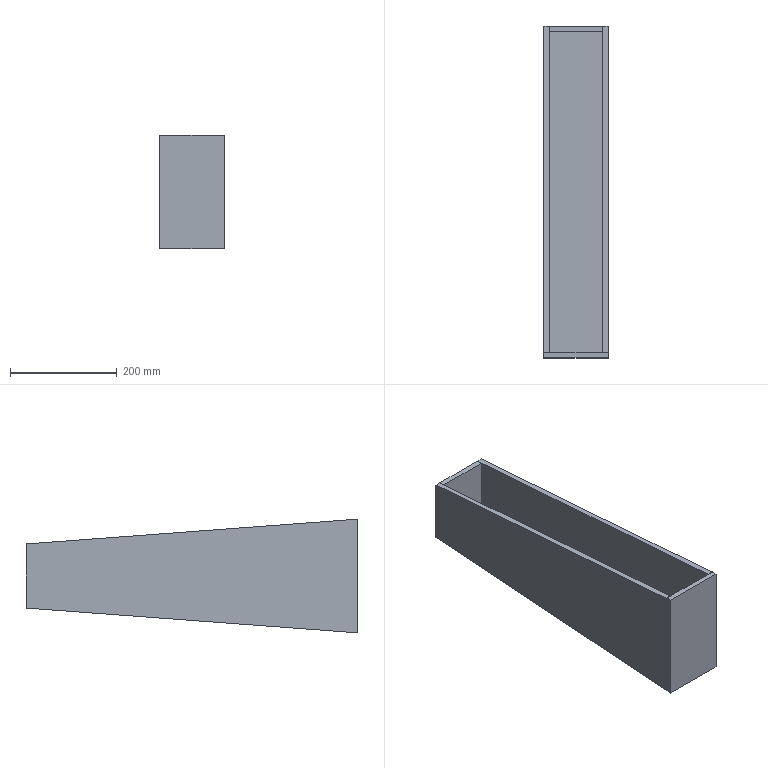Part | STEP file | 1 solid | 20 faces | box 120 x 620.836 x 212.718 mm | volume 2999336 mm3 | plane 20
STEP:
#1=CARTESIAN_POINT('',(0.,0.,0.));
#2=DIRECTION('',(0.,0.,1.));
#3=DIRECTION('',(1.,0.,0.));
#4=AXIS2_PLACEMENT_3D('',#1,#2,#3);
#5=CARTESIAN_POINT('',(-590.,-180.836,-60.));
#6=VERTEX_POINT('',#5);
#7=CARTESIAN_POINT('',(-490.,-180.836,-60.));
#8=VERTEX_POINT('',#7);
#9=CARTESIAN_POINT('',(0.,-180.836,-60.));
#10=DIRECTION('',(1.,0.,0.));
#11=VECTOR('',#10,1.);
#12=LINE('',#9,#11);
#13=CARTESIAN_POINT('',(0.,0.,-60.));
#14=DIRECTION('',(0.,0.,1.));
#15=DIRECTION('',(1.,0.,0.));
#16=AXIS2_PLACEMENT_3D('',#13,#14,#15);
#17=PLANE('',#16);
#18=CARTESIAN_POINT('',(0.,-180.836));
#19=DIRECTION('',(1.,0.));
#20=VECTOR('',#19,1.);
#21=LINE('',#18,#20);
#22=(GEOMETRIC_REPRESENTATION_CONTEXT(2)PARAMETRIC_REPRESENTATION_CONTEXT()REPRESENTATION_CONTEXT('',''));
#23=DEFINITIONAL_REPRESENTATION('',(#21),#22);
#24=PCURVE('',#17,#23);
#25=CARTESIAN_POINT('',(0.,-180.836,0.));
#26=DIRECTION('',(0.,-1.,0.));
#27=DIRECTION('',(1.,0.,0.));
#28=AXIS2_PLACEMENT_3D('',#25,#26,#27);
#29=PLANE('',#28);
#30=CARTESIAN_POINT('',(0.,-60.));
#31=DIRECTION('',(1.,0.));
#32=VECTOR('',#31,1.);
#33=LINE('',#30,#32);
#34=(GEOMETRIC_REPRESENTATION_CONTEXT(2)PARAMETRIC_REPRESENTATION_CONTEXT()REPRESENTATION_CONTEXT('',''));
#35=DEFINITIONAL_REPRESENTATION('',(#33),#34);
#36=PCURVE('',#29,#35);
#37=SURFACE_CURVE('',#12,(#24,#36),.PCURVE_S1.);
#38=EDGE_CURVE('',#6,#8,#37,.T.);
#39=ORIENTED_EDGE('',*,*,#38,.F.);
#40=CARTESIAN_POINT('',(-590.,430.,-60.));
#41=VERTEX_POINT('',#40);
#42=CARTESIAN_POINT('',(-590.,-190.836,-60.));
#43=DIRECTION('',(0.,-1.,0.));
#44=VECTOR('',#43,1.);
#45=LINE('',#42,#44);
#46=CARTESIAN_POINT('',(-590.,-190.836));
#47=DIRECTION('',(0.,-1.));
#48=VECTOR('',#47,1.);
#49=LINE('',#46,#48);
#50=(GEOMETRIC_REPRESENTATION_CONTEXT(2)PARAMETRIC_REPRESENTATION_CONTEXT()REPRESENTATION_CONTEXT('',''));
#51=DEFINITIONAL_REPRESENTATION('',(#49),#50);
#52=PCURVE('',#17,#51);
#53=CARTESIAN_POINT('',(-590.,0.,0.));
#54=DIRECTION('',(-1.,0.,0.));
#55=DIRECTION('',(0.,0.,-1.));
#56=AXIS2_PLACEMENT_3D('',#53,#54,#55);
#57=PLANE('',#56);
#58=CARTESIAN_POINT('',(60.,190.836));
#59=DIRECTION('',(0.,1.));
#60=VECTOR('',#59,1.);
#61=LINE('',#58,#60);
#62=(GEOMETRIC_REPRESENTATION_CONTEXT(2)PARAMETRIC_REPRESENTATION_CONTEXT()REPRESENTATION_CONTEXT('',''));
#63=DEFINITIONAL_REPRESENTATION('',(#61),#62);
#64=PCURVE('',#57,#63);
#65=SURFACE_CURVE('',#45,(#52,#64),.PCURVE_S1.);
#66=EDGE_CURVE('',#41,#6,#65,.T.);
#67=ORIENTED_EDGE('',*,*,#66,.F.);
#68=CARTESIAN_POINT('',(-490.,430.,-60.));
#69=VERTEX_POINT('',#68);
#70=CARTESIAN_POINT('',(0.,430.,-60.));
#71=DIRECTION('',(1.,0.,0.));
#72=VECTOR('',#71,1.);
#73=LINE('',#70,#72);
#74=CARTESIAN_POINT('',(0.,430.));
#75=DIRECTION('',(1.,0.));
#76=VECTOR('',#75,1.);
#77=LINE('',#74,#76);
#78=(GEOMETRIC_REPRESENTATION_CONTEXT(2)PARAMETRIC_REPRESENTATION_CONTEXT()REPRESENTATION_CONTEXT('',''));
#79=DEFINITIONAL_REPRESENTATION('',(#77),#78);
#80=PCURVE('',#17,#79);
#81=CARTESIAN_POINT('',(480.,430.,-60.));
#82=DIRECTION('',(0.,-1.,0.));
#83=DIRECTION('',(1.,0.,0.));
#84=AXIS2_PLACEMENT_3D('',#81,#82,#83);
#85=PLANE('',#84);
#86=CARTESIAN_POINT('',(-480.,0.));
#87=DIRECTION('',(1.,0.));
#88=VECTOR('',#87,1.);
#89=LINE('',#86,#88);
#90=(GEOMETRIC_REPRESENTATION_CONTEXT(2)PARAMETRIC_REPRESENTATION_CONTEXT()REPRESENTATION_CONTEXT('',''));
#91=DEFINITIONAL_REPRESENTATION('',(#89),#90);
#92=PCURVE('',#85,#91);
#93=SURFACE_CURVE('',#73,(#80,#92),.PCURVE_S1.);
#94=EDGE_CURVE('',#41,#69,#93,.T.);
#95=ORIENTED_EDGE('',*,*,#94,.T.);
#96=CARTESIAN_POINT('',(-490.,-190.836,-60.));
#97=DIRECTION('',(0.,-1.,0.));
#98=VECTOR('',#97,1.);
#99=LINE('',#96,#98);
#100=CARTESIAN_POINT('',(-490.,-190.836));
#101=DIRECTION('',(0.,-1.));
#102=VECTOR('',#101,1.);
#103=LINE('',#100,#102);
#104=(GEOMETRIC_REPRESENTATION_CONTEXT(2)PARAMETRIC_REPRESENTATION_CONTEXT()REPRESENTATION_CONTEXT('',''));
#105=DEFINITIONAL_REPRESENTATION('',(#103),#104);
#106=PCURVE('',#17,#105);
#107=CARTESIAN_POINT('',(-490.,0.,0.));
#108=DIRECTION('',(1.,0.,0.));
#109=DIRECTION('',(0.,0.,-1.));
#110=AXIS2_PLACEMENT_3D('',#107,#108,#109);
#111=PLANE('',#110);
#112=CARTESIAN_POINT('',(60.,-190.836));
#113=DIRECTION('',(0.,-1.));
#114=VECTOR('',#113,1.);
#115=LINE('',#112,#114);
#116=(GEOMETRIC_REPRESENTATION_CONTEXT(2)PARAMETRIC_REPRESENTATION_CONTEXT()REPRESENTATION_CONTEXT('',''));
#117=DEFINITIONAL_REPRESENTATION('',(#115),#116);
#118=PCURVE('',#111,#117);
#119=SURFACE_CURVE('',#99,(#106,#118),.PCURVE_S1.);
#120=EDGE_CURVE('',#69,#8,#119,.T.);
#121=ORIENTED_EDGE('',*,*,#120,.T.);
#122=EDGE_LOOP('',(#39,#67,#95,#121));
#123=FACE_BOUND('',#122,.T.);
#124=ADVANCED_FACE('',(#123),#17,.F.);
#125=CARTESIAN_POINT('',(-490.,-180.836,105.612));
#126=VERTEX_POINT('',#125);
#127=CARTESIAN_POINT('',(-490.,-180.836,-50.));
#128=VERTEX_POINT('',#127);
#129=CARTESIAN_POINT('',(-490.,-180.836,60.));
#130=DIRECTION('',(0.,0.,-1.));
#131=VECTOR('',#130,1.);
#132=LINE('',#129,#131);
#133=CARTESIAN_POINT('',(-490.,0.,60.));
#134=DIRECTION('',(1.,0.,0.));
#135=DIRECTION('',(0.,0.,-1.));
#136=AXIS2_PLACEMENT_3D('',#133,#134,#135);
#137=PLANE('',#136);
#138=CARTESIAN_POINT('',(0.,-180.836));
#139=DIRECTION('',(1.,0.));
#140=VECTOR('',#139,1.);
#141=LINE('',#138,#140);
#142=(GEOMETRIC_REPRESENTATION_CONTEXT(2)PARAMETRIC_REPRESENTATION_CONTEXT()REPRESENTATION_CONTEXT('',''));
#143=DEFINITIONAL_REPRESENTATION('',(#141),#142);
#144=PCURVE('',#137,#143);
#145=CARTESIAN_POINT('',(-600.,-180.836,60.));
#146=DIRECTION('',(0.,1.,0.));
#147=DIRECTION('',(-1.,0.,0.));
#148=AXIS2_PLACEMENT_3D('',#145,#146,#147);
#149=PLANE('',#148);
#150=CARTESIAN_POINT('',(-110.,0.));
#151=DIRECTION('',(0.,-1.));
#152=VECTOR('',#151,1.);
#153=LINE('',#150,#152);
#154=(GEOMETRIC_REPRESENTATION_CONTEXT(2)PARAMETRIC_REPRESENTATION_CONTEXT()REPRESENTATION_CONTEXT('',''));
#155=DEFINITIONAL_REPRESENTATION('',(#153),#154);
#156=PCURVE('',#149,#155);
#157=SURFACE_CURVE('',#132,(#144,#156),.PCURVE_S1.);
#158=EDGE_CURVE('',#126,#128,#157,.T.);
#159=ORIENTED_EDGE('',*,*,#158,.F.);
#160=CARTESIAN_POINT('',(-490.,430.,60.));
#161=VERTEX_POINT('',#160);
#162=CARTESIAN_POINT('',(-490.,430.,60.));
#163=DIRECTION('',(0.,0.9972,-0.07446));
#164=VECTOR('',#163,1.);
#165=LINE('',#162,#164);
#166=CARTESIAN_POINT('',(0.,430.));
#167=DIRECTION('',(0.07446,0.9972));
#168=VECTOR('',#167,1.);
#169=LINE('',#166,#168);
#170=(GEOMETRIC_REPRESENTATION_CONTEXT(2)PARAMETRIC_REPRESENTATION_CONTEXT()REPRESENTATION_CONTEXT('',''));
#171=DEFINITIONAL_REPRESENTATION('',(#169),#170);
#172=PCURVE('',#137,#171);
#173=CARTESIAN_POINT('',(-490.,430.,60.));
#174=DIRECTION('',(0.,0.07446,0.9972));
#175=DIRECTION('',(0.,-0.9972,0.07446));
#176=AXIS2_PLACEMENT_3D('',#173,#174,#175);
#177=PLANE('',#176);
#178=CARTESIAN_POINT('',(0.,0.));
#179=DIRECTION('',(-1.,0.));
#180=VECTOR('',#179,1.);
#181=LINE('',#178,#180);
#182=(GEOMETRIC_REPRESENTATION_CONTEXT(2)PARAMETRIC_REPRESENTATION_CONTEXT()REPRESENTATION_CONTEXT('',''));
#183=DEFINITIONAL_REPRESENTATION('',(#181),#182);
#184=PCURVE('',#177,#183);
#185=SURFACE_CURVE('',#165,(#172,#184),.PCURVE_S1.);
#186=EDGE_CURVE('',#126,#161,#185,.T.);
#187=ORIENTED_EDGE('',*,*,#186,.T.);
#188=CARTESIAN_POINT('',(-490.,420.,60.));
#189=VERTEX_POINT('',#188);
#190=CARTESIAN_POINT('',(-490.,-190.836,60.));
#191=DIRECTION('',(0.,-1.,0.));
#192=VECTOR('',#191,1.);
#193=LINE('',#190,#192);
#194=CARTESIAN_POINT('',(0.,-190.836));
#195=DIRECTION('',(0.,-1.));
#196=VECTOR('',#195,1.);
#197=LINE('',#194,#196);
#198=(GEOMETRIC_REPRESENTATION_CONTEXT(2)PARAMETRIC_REPRESENTATION_CONTEXT()REPRESENTATION_CONTEXT('',''));
#199=DEFINITIONAL_REPRESENTATION('',(#197),#198);
#200=PCURVE('',#137,#199);
#201=CARTESIAN_POINT('',(0.,0.,60.));
#202=DIRECTION('',(0.,0.,1.));
#203=DIRECTION('',(1.,0.,0.));
#204=AXIS2_PLACEMENT_3D('',#201,#202,#203);
#205=PLANE('',#204);
#206=CARTESIAN_POINT('',(-490.,-190.836));
#207=DIRECTION('',(0.,-1.));
#208=VECTOR('',#207,1.);
#209=LINE('',#206,#208);
#210=(GEOMETRIC_REPRESENTATION_CONTEXT(2)PARAMETRIC_REPRESENTATION_CONTEXT()REPRESENTATION_CONTEXT('',''));
#211=DEFINITIONAL_REPRESENTATION('',(#209),#210);
#212=PCURVE('',#205,#211);
#213=SURFACE_CURVE('',#193,(#200,#212),.PCURVE_S1.);
#214=EDGE_CURVE('',#161,#189,#213,.T.);
#215=ORIENTED_EDGE('',*,*,#214,.T.);
#216=CARTESIAN_POINT('',(-490.,420.,-50.));
#217=VERTEX_POINT('',#216);
#218=CARTESIAN_POINT('',(-490.,420.,60.));
#219=DIRECTION('',(0.,0.,-1.));
#220=VECTOR('',#219,1.);
#221=LINE('',#218,#220);
#222=CARTESIAN_POINT('',(0.,420.));
#223=DIRECTION('',(1.,0.));
#224=VECTOR('',#223,1.);
#225=LINE('',#222,#224);
#226=(GEOMETRIC_REPRESENTATION_CONTEXT(2)PARAMETRIC_REPRESENTATION_CONTEXT()REPRESENTATION_CONTEXT('',''));
#227=DEFINITIONAL_REPRESENTATION('',(#225),#226);
#228=PCURVE('',#137,#227);
#229=CARTESIAN_POINT('',(480.,420.,-60.));
#230=DIRECTION('',(0.,-1.,0.));
#231=DIRECTION('',(1.,0.,0.));
#232=AXIS2_PLACEMENT_3D('',#229,#230,#231);
#233=PLANE('',#232);
#234=CARTESIAN_POINT('',(-970.,120.));
#235=DIRECTION('',(0.,-1.));
#236=VECTOR('',#235,1.);
#237=LINE('',#234,#236);
#238=(GEOMETRIC_REPRESENTATION_CONTEXT(2)PARAMETRIC_REPRESENTATION_CONTEXT()REPRESENTATION_CONTEXT('',''));
#239=DEFINITIONAL_REPRESENTATION('',(#237),#238);
#240=PCURVE('',#233,#239);
#241=SURFACE_CURVE('',#221,(#228,#240),.PCURVE_S1.);
#242=EDGE_CURVE('',#189,#217,#241,.T.);
#243=ORIENTED_EDGE('',*,*,#242,.T.);
#244=CARTESIAN_POINT('',(-490.,0.,-50.));
#245=DIRECTION('',(0.,-1.,0.));
#246=VECTOR('',#245,1.);
#247=LINE('',#244,#246);
#248=CARTESIAN_POINT('',(110.,0.));
#249=DIRECTION('',(0.,-1.));
#250=VECTOR('',#249,1.);
#251=LINE('',#248,#250);
#252=(GEOMETRIC_REPRESENTATION_CONTEXT(2)PARAMETRIC_REPRESENTATION_CONTEXT()REPRESENTATION_CONTEXT('',''));
#253=DEFINITIONAL_REPRESENTATION('',(#251),#252);
#254=PCURVE('',#137,#253);
#255=CARTESIAN_POINT('',(0.,0.,-50.));
#256=DIRECTION('',(0.,0.,1.));
#257=DIRECTION('',(1.,0.,0.));
#258=AXIS2_PLACEMENT_3D('',#255,#256,#257);
#259=PLANE('',#258);
#260=CARTESIAN_POINT('',(-490.,0.));
#261=DIRECTION('',(0.,-1.));
#262=VECTOR('',#261,1.);
#263=LINE('',#260,#262);
#264=(GEOMETRIC_REPRESENTATION_CONTEXT(2)PARAMETRIC_REPRESENTATION_CONTEXT()REPRESENTATION_CONTEXT('',''));
#265=DEFINITIONAL_REPRESENTATION('',(#263),#264);
#266=PCURVE('',#259,#265);
#267=SURFACE_CURVE('',#247,(#254,#266),.PCURVE_S1.);
#268=EDGE_CURVE('',#217,#128,#267,.T.);
#269=ORIENTED_EDGE('',*,*,#268,.T.);
#270=EDGE_LOOP('',(#159,#187,#215,#243,#269));
#271=FACE_BOUND('',#270,.T.);
#272=ADVANCED_FACE('',(#271),#137,.F.);
#273=CARTESIAN_POINT('',(-590.,-180.836,105.612));
#274=VERTEX_POINT('',#273);
#275=CARTESIAN_POINT('',(-590.,430.,60.));
#276=VERTEX_POINT('',#275);
#277=CARTESIAN_POINT('',(-590.,430.,60.));
#278=DIRECTION('',(0.,0.9972,-0.07446));
#279=VECTOR('',#278,1.);
#280=LINE('',#277,#279);
#281=CARTESIAN_POINT('',(-590.,0.,60.));
#282=DIRECTION('',(1.,0.,0.));
#283=DIRECTION('',(0.,0.,-1.));
#284=AXIS2_PLACEMENT_3D('',#281,#282,#283);
#285=PLANE('',#284);
#286=CARTESIAN_POINT('',(0.,430.));
#287=DIRECTION('',(0.07446,0.9972));
#288=VECTOR('',#287,1.);
#289=LINE('',#286,#288);
#290=(GEOMETRIC_REPRESENTATION_CONTEXT(2)PARAMETRIC_REPRESENTATION_CONTEXT()REPRESENTATION_CONTEXT('',''));
#291=DEFINITIONAL_REPRESENTATION('',(#289),#290);
#292=PCURVE('',#285,#291);
#293=CARTESIAN_POINT('',(-590.,430.,60.));
#294=DIRECTION('',(0.,0.07446,0.9972));
#295=DIRECTION('',(0.,-0.9972,0.07446));
#296=AXIS2_PLACEMENT_3D('',#293,#294,#295);
#297=PLANE('',#296);
#298=CARTESIAN_POINT('',(0.,0.));
#299=DIRECTION('',(-1.,0.));
#300=VECTOR('',#299,1.);
#301=LINE('',#298,#300);
#302=(GEOMETRIC_REPRESENTATION_CONTEXT(2)PARAMETRIC_REPRESENTATION_CONTEXT()REPRESENTATION_CONTEXT('',''));
#303=DEFINITIONAL_REPRESENTATION('',(#301),#302);
#304=PCURVE('',#297,#303);
#305=SURFACE_CURVE('',#280,(#292,#304),.PCURVE_S1.);
#306=EDGE_CURVE('',#274,#276,#305,.T.);
#307=ORIENTED_EDGE('',*,*,#306,.F.);
#308=CARTESIAN_POINT('',(-590.,-180.836,-50.));
#309=VERTEX_POINT('',#308);
#310=CARTESIAN_POINT('',(-590.,-180.836,60.));
#311=DIRECTION('',(0.,0.,1.));
#312=VECTOR('',#311,1.);
#313=LINE('',#310,#312);
#314=CARTESIAN_POINT('',(0.,-180.836));
#315=DIRECTION('',(-1.,0.));
#316=VECTOR('',#315,1.);
#317=LINE('',#314,#316);
#318=(GEOMETRIC_REPRESENTATION_CONTEXT(2)PARAMETRIC_REPRESENTATION_CONTEXT()REPRESENTATION_CONTEXT('',''));
#319=DEFINITIONAL_REPRESENTATION('',(#317),#318);
#320=PCURVE('',#285,#319);
#321=CARTESIAN_POINT('',(-10.,0.));
#322=DIRECTION('',(0.,1.));
#323=VECTOR('',#322,1.);
#324=LINE('',#321,#323);
#325=(GEOMETRIC_REPRESENTATION_CONTEXT(2)PARAMETRIC_REPRESENTATION_CONTEXT()REPRESENTATION_CONTEXT('',''));
#326=DEFINITIONAL_REPRESENTATION('',(#324),#325);
#327=PCURVE('',#149,#326);
#328=SURFACE_CURVE('',#313,(#320,#327),.PCURVE_S1.);
#329=EDGE_CURVE('',#309,#274,#328,.T.);
#330=ORIENTED_EDGE('',*,*,#329,.F.);
#331=CARTESIAN_POINT('',(-590.,420.,-50.));
#332=VERTEX_POINT('',#331);
#333=CARTESIAN_POINT('',(-590.,0.,-50.));
#334=DIRECTION('',(0.,-1.,0.));
#335=VECTOR('',#334,1.);
#336=LINE('',#333,#335);
#337=CARTESIAN_POINT('',(110.,0.));
#338=DIRECTION('',(0.,-1.));
#339=VECTOR('',#338,1.);
#340=LINE('',#337,#339);
#341=(GEOMETRIC_REPRESENTATION_CONTEXT(2)PARAMETRIC_REPRESENTATION_CONTEXT()REPRESENTATION_CONTEXT('',''));
#342=DEFINITIONAL_REPRESENTATION('',(#340),#341);
#343=PCURVE('',#285,#342);
#344=CARTESIAN_POINT('',(-590.,0.));
#345=DIRECTION('',(0.,-1.));
#346=VECTOR('',#345,1.);
#347=LINE('',#344,#346);
#348=(GEOMETRIC_REPRESENTATION_CONTEXT(2)PARAMETRIC_REPRESENTATION_CONTEXT()REPRESENTATION_CONTEXT('',''));
#349=DEFINITIONAL_REPRESENTATION('',(#347),#348);
#350=PCURVE('',#259,#349);
#351=SURFACE_CURVE('',#336,(#343,#350),.PCURVE_S1.);
#352=EDGE_CURVE('',#332,#309,#351,.T.);
#353=ORIENTED_EDGE('',*,*,#352,.F.);
#354=CARTESIAN_POINT('',(-590.,420.,60.));
#355=VERTEX_POINT('',#354);
#356=CARTESIAN_POINT('',(-590.,420.,60.));
#357=DIRECTION('',(0.,0.,-1.));
#358=VECTOR('',#357,1.);
#359=LINE('',#356,#358);
#360=CARTESIAN_POINT('',(0.,420.));
#361=DIRECTION('',(1.,0.));
#362=VECTOR('',#361,1.);
#363=LINE('',#360,#362);
#364=(GEOMETRIC_REPRESENTATION_CONTEXT(2)PARAMETRIC_REPRESENTATION_CONTEXT()REPRESENTATION_CONTEXT('',''));
#365=DEFINITIONAL_REPRESENTATION('',(#363),#364);
#366=PCURVE('',#285,#365);
#367=CARTESIAN_POINT('',(-1070.,120.));
#368=DIRECTION('',(0.,-1.));
#369=VECTOR('',#368,1.);
#370=LINE('',#367,#369);
#371=(GEOMETRIC_REPRESENTATION_CONTEXT(2)PARAMETRIC_REPRESENTATION_CONTEXT()REPRESENTATION_CONTEXT('',''));
#372=DEFINITIONAL_REPRESENTATION('',(#370),#371);
#373=PCURVE('',#233,#372);
#374=SURFACE_CURVE('',#359,(#366,#373),.PCURVE_S1.);
#375=EDGE_CURVE('',#355,#332,#374,.T.);
#376=ORIENTED_EDGE('',*,*,#375,.F.);
#377=CARTESIAN_POINT('',(-590.,-190.836,60.));
#378=DIRECTION('',(0.,-1.,0.));
#379=VECTOR('',#378,1.);
#380=LINE('',#377,#379);
#381=CARTESIAN_POINT('',(0.,-190.836));
#382=DIRECTION('',(0.,-1.));
#383=VECTOR('',#382,1.);
#384=LINE('',#381,#383);
#385=(GEOMETRIC_REPRESENTATION_CONTEXT(2)PARAMETRIC_REPRESENTATION_CONTEXT()REPRESENTATION_CONTEXT('',''));
#386=DEFINITIONAL_REPRESENTATION('',(#384),#385);
#387=PCURVE('',#285,#386);
#388=CARTESIAN_POINT('',(-590.,-190.836));
#389=DIRECTION('',(0.,-1.));
#390=VECTOR('',#389,1.);
#391=LINE('',#388,#390);
#392=(GEOMETRIC_REPRESENTATION_CONTEXT(2)PARAMETRIC_REPRESENTATION_CONTEXT()REPRESENTATION_CONTEXT('',''));
#393=DEFINITIONAL_REPRESENTATION('',(#391),#392);
#394=PCURVE('',#205,#393);
#395=SURFACE_CURVE('',#380,(#387,#394),.PCURVE_S1.);
#396=EDGE_CURVE('',#276,#355,#395,.T.);
#397=ORIENTED_EDGE('',*,*,#396,.F.);
#398=EDGE_LOOP('',(#307,#330,#353,#376,#397));
#399=FACE_BOUND('',#398,.T.);
#400=ADVANCED_FACE('',(#399),#285,.T.);
#401=ORIENTED_EDGE('',*,*,#186,.F.);
#402=CARTESIAN_POINT('',(-480.,-180.836,105.612));
#403=VERTEX_POINT('',#402);
#404=CARTESIAN_POINT('',(-490.,-180.836,105.612));
#405=DIRECTION('',(1.,0.,0.));
#406=VECTOR('',#405,1.);
#407=LINE('',#404,#406);
#408=CARTESIAN_POINT('',(612.537,0.));
#409=DIRECTION('',(0.,1.));
#410=VECTOR('',#409,1.);
#411=LINE('',#408,#410);
#412=(GEOMETRIC_REPRESENTATION_CONTEXT(2)PARAMETRIC_REPRESENTATION_CONTEXT()REPRESENTATION_CONTEXT('',''));
#413=DEFINITIONAL_REPRESENTATION('',(#411),#412);
#414=PCURVE('',#177,#413);
#415=CARTESIAN_POINT('',(-110.,45.612));
#416=DIRECTION('',(-1.,0.));
#417=VECTOR('',#416,1.);
#418=LINE('',#415,#417);
#419=(GEOMETRIC_REPRESENTATION_CONTEXT(2)PARAMETRIC_REPRESENTATION_CONTEXT()REPRESENTATION_CONTEXT('',''));
#420=DEFINITIONAL_REPRESENTATION('',(#418),#419);
#421=PCURVE('',#149,#420);
#422=SURFACE_CURVE('',#407,(#414,#421),.PCURVE_S1.);
#423=EDGE_CURVE('',#126,#403,#422,.T.);
#424=ORIENTED_EDGE('',*,*,#423,.T.);
#425=CARTESIAN_POINT('',(-480.,430.,60.));
#426=VERTEX_POINT('',#425);
#427=CARTESIAN_POINT('',(-480.,430.,60.));
#428=DIRECTION('',(0.,0.9972,-0.07446));
#429=VECTOR('',#428,1.);
#430=LINE('',#427,#429);
#431=CARTESIAN_POINT('',(0.,10.));
#432=DIRECTION('',(-1.,0.));
#433=VECTOR('',#432,1.);
#434=LINE('',#431,#433);
#435=(GEOMETRIC_REPRESENTATION_CONTEXT(2)PARAMETRIC_REPRESENTATION_CONTEXT()REPRESENTATION_CONTEXT('',''));
#436=DEFINITIONAL_REPRESENTATION('',(#434),#435);
#437=PCURVE('',#177,#436);
#438=CARTESIAN_POINT('',(-480.,0.,60.));
#439=DIRECTION('',(1.,0.,0.));
#440=DIRECTION('',(0.,0.,-1.));
#441=AXIS2_PLACEMENT_3D('',#438,#439,#440);
#442=PLANE('',#441);
#443=CARTESIAN_POINT('',(0.,430.));
#444=DIRECTION('',(0.07446,0.9972));
#445=VECTOR('',#444,1.);
#446=LINE('',#443,#445);
#447=(GEOMETRIC_REPRESENTATION_CONTEXT(2)PARAMETRIC_REPRESENTATION_CONTEXT()REPRESENTATION_CONTEXT('',''));
#448=DEFINITIONAL_REPRESENTATION('',(#446),#447);
#449=PCURVE('',#442,#448);
#450=SURFACE_CURVE('',#430,(#437,#449),.PCURVE_S1.);
#451=EDGE_CURVE('',#403,#426,#450,.T.);
#452=ORIENTED_EDGE('',*,*,#451,.T.);
#453=CARTESIAN_POINT('',(-490.,430.,60.));
#454=DIRECTION('',(1.,0.,0.));
#455=VECTOR('',#454,1.);
#456=LINE('',#453,#455);
#457=CARTESIAN_POINT('',(0.,0.));
#458=DIRECTION('',(0.,1.));
#459=VECTOR('',#458,1.);
#460=LINE('',#457,#459);
#461=(GEOMETRIC_REPRESENTATION_CONTEXT(2)PARAMETRIC_REPRESENTATION_CONTEXT()REPRESENTATION_CONTEXT('',''));
#462=DEFINITIONAL_REPRESENTATION('',(#460),#461);
#463=PCURVE('',#177,#462);
#464=CARTESIAN_POINT('',(-970.,120.));
#465=DIRECTION('',(1.,0.));
#466=VECTOR('',#465,1.);
#467=LINE('',#464,#466);
#468=(GEOMETRIC_REPRESENTATION_CONTEXT(2)PARAMETRIC_REPRESENTATION_CONTEXT()REPRESENTATION_CONTEXT('',''));
#469=DEFINITIONAL_REPRESENTATION('',(#467),#468);
#470=PCURVE('',#85,#469);
#471=SURFACE_CURVE('',#456,(#463,#470),.PCURVE_S1.);
#472=EDGE_CURVE('',#161,#426,#471,.T.);
#473=ORIENTED_EDGE('',*,*,#472,.F.);
#474=EDGE_LOOP('',(#401,#424,#452,#473));
#475=FACE_BOUND('',#474,.T.);
#476=ADVANCED_FACE('',(#475),#177,.T.);
#477=CARTESIAN_POINT('',(-590.,-180.836,-105.612));
#478=VERTEX_POINT('',#477);
#479=CARTESIAN_POINT('',(-590.,430.,-60.));
#480=DIRECTION('',(0.,0.9972,0.07446));
#481=VECTOR('',#480,1.);
#482=LINE('',#479,#481);
#483=CARTESIAN_POINT('',(-590.,430.,-60.));
#484=DIRECTION('',(0.,0.07446,-0.9972));
#485=DIRECTION('',(0.,-0.9972,-0.07446));
#486=AXIS2_PLACEMENT_3D('',#483,#484,#485);
#487=PLANE('',#486);
#488=CARTESIAN_POINT('',(0.,0.));
#489=DIRECTION('',(-1.,0.));
#490=VECTOR('',#489,1.);
#491=LINE('',#488,#490);
#492=(GEOMETRIC_REPRESENTATION_CONTEXT(2)PARAMETRIC_REPRESENTATION_CONTEXT()REPRESENTATION_CONTEXT('',''));
#493=DEFINITIONAL_REPRESENTATION('',(#491),#492);
#494=PCURVE('',#487,#493);
#495=CARTESIAN_POINT('',(60.,-430.));
#496=DIRECTION('',(-0.07446,-0.9972));
#497=VECTOR('',#496,1.);
#498=LINE('',#495,#497);
#499=(GEOMETRIC_REPRESENTATION_CONTEXT(2)PARAMETRIC_REPRESENTATION_CONTEXT()REPRESENTATION_CONTEXT('',''));
#500=DEFINITIONAL_REPRESENTATION('',(#498),#499);
#501=PCURVE('',#57,#500);
#502=SURFACE_CURVE('',#482,(#494,#501),.PCURVE_S1.);
#503=EDGE_CURVE('',#478,#41,#502,.T.);
#504=ORIENTED_EDGE('',*,*,#503,.F.);
#505=CARTESIAN_POINT('',(-600.,-180.836,-105.612));
#506=VERTEX_POINT('',#505);
#507=CARTESIAN_POINT('',(-590.,-180.836,-105.612));
#508=DIRECTION('',(-1.,0.,0.));
#509=VECTOR('',#508,1.);
#510=LINE('',#507,#509);
#511=CARTESIAN_POINT('',(612.537,0.));
#512=DIRECTION('',(0.,1.));
#513=VECTOR('',#512,1.);
#514=LINE('',#511,#513);
#515=(GEOMETRIC_REPRESENTATION_CONTEXT(2)PARAMETRIC_REPRESENTATION_CONTEXT()REPRESENTATION_CONTEXT('',''));
#516=DEFINITIONAL_REPRESENTATION('',(#514),#515);
#517=PCURVE('',#487,#516);
#518=CARTESIAN_POINT('',(-590.,-105.612));
#519=DIRECTION('',(-1.,0.));
#520=VECTOR('',#519,1.);
#521=LINE('',#518,#520);
#522=(GEOMETRIC_REPRESENTATION_CONTEXT(2)PARAMETRIC_REPRESENTATION_CONTEXT()REPRESENTATION_CONTEXT('',''));
#523=DEFINITIONAL_REPRESENTATION('',(#521),#522);
#524=PCURVE('',#29,#523);
#525=SURFACE_CURVE('',#510,(#517,#524),.PCURVE_S1.);
#526=EDGE_CURVE('',#478,#506,#525,.T.);
#527=ORIENTED_EDGE('',*,*,#526,.T.);
#528=CARTESIAN_POINT('',(-600.,430.,-60.));
#529=VERTEX_POINT('',#528);
#530=CARTESIAN_POINT('',(-600.,430.,-60.));
#531=DIRECTION('',(0.,0.9972,0.07446));
#532=VECTOR('',#531,1.);
#533=LINE('',#530,#532);
#534=CARTESIAN_POINT('',(0.,10.));
#535=DIRECTION('',(-1.,0.));
#536=VECTOR('',#535,1.);
#537=LINE('',#534,#536);
#538=(GEOMETRIC_REPRESENTATION_CONTEXT(2)PARAMETRIC_REPRESENTATION_CONTEXT()REPRESENTATION_CONTEXT('',''));
#539=DEFINITIONAL_REPRESENTATION('',(#537),#538);
#540=PCURVE('',#487,#539);
#541=CARTESIAN_POINT('',(-600.,0.,60.));
#542=DIRECTION('',(1.,0.,0.));
#543=DIRECTION('',(0.,0.,-1.));
#544=AXIS2_PLACEMENT_3D('',#541,#542,#543);
#545=PLANE('',#544);
#546=CARTESIAN_POINT('',(120.,430.));
#547=DIRECTION('',(-0.07446,0.9972));
#548=VECTOR('',#547,1.);
#549=LINE('',#546,#548);
#550=(GEOMETRIC_REPRESENTATION_CONTEXT(2)PARAMETRIC_REPRESENTATION_CONTEXT()REPRESENTATION_CONTEXT('',''));
#551=DEFINITIONAL_REPRESENTATION('',(#549),#550);
#552=PCURVE('',#545,#551);
#553=SURFACE_CURVE('',#533,(#540,#552),.PCURVE_S1.);
#554=EDGE_CURVE('',#506,#529,#553,.T.);
#555=ORIENTED_EDGE('',*,*,#554,.T.);
#556=CARTESIAN_POINT('',(-590.,430.,-60.));
#557=DIRECTION('',(-1.,0.,0.));
#558=VECTOR('',#557,1.);
#559=LINE('',#556,#558);
#560=CARTESIAN_POINT('',(0.,0.));
#561=DIRECTION('',(0.,1.));
#562=VECTOR('',#561,1.);
#563=LINE('',#560,#562);
#564=(GEOMETRIC_REPRESENTATION_CONTEXT(2)PARAMETRIC_REPRESENTATION_CONTEXT()REPRESENTATION_CONTEXT('',''));
#565=DEFINITIONAL_REPRESENTATION('',(#563),#564);
#566=PCURVE('',#487,#565);
#567=CARTESIAN_POINT('',(-1070.,0.));
#568=DIRECTION('',(-1.,0.));
#569=VECTOR('',#568,1.);
#570=LINE('',#567,#569);
#571=(GEOMETRIC_REPRESENTATION_CONTEXT(2)PARAMETRIC_REPRESENTATION_CONTEXT()REPRESENTATION_CONTEXT('',''));
#572=DEFINITIONAL_REPRESENTATION('',(#570),#571);
#573=PCURVE('',#85,#572);
#574=SURFACE_CURVE('',#559,(#566,#573),.PCURVE_S1.);
#575=EDGE_CURVE('',#41,#529,#574,.T.);
#576=ORIENTED_EDGE('',*,*,#575,.F.);
#577=EDGE_LOOP('',(#504,#527,#555,#576));
#578=FACE_BOUND('',#577,.T.);
#579=ADVANCED_FACE('',(#578),#487,.T.);
#580=CARTESIAN_POINT('',(-590.,-180.836,0.));
#581=DIRECTION('',(0.,0.,1.));
#582=VECTOR('',#581,1.);
#583=LINE('',#580,#582);
#584=CARTESIAN_POINT('',(0.,180.836));
#585=DIRECTION('',(-1.,0.));
#586=VECTOR('',#585,1.);
#587=LINE('',#584,#586);
#588=(GEOMETRIC_REPRESENTATION_CONTEXT(2)PARAMETRIC_REPRESENTATION_CONTEXT()REPRESENTATION_CONTEXT('',''));
#589=DEFINITIONAL_REPRESENTATION('',(#587),#588);
#590=PCURVE('',#57,#589);
#591=CARTESIAN_POINT('',(-590.,0.));
#592=DIRECTION('',(0.,1.));
#593=VECTOR('',#592,1.);
#594=LINE('',#591,#593);
#595=(GEOMETRIC_REPRESENTATION_CONTEXT(2)PARAMETRIC_REPRESENTATION_CONTEXT()REPRESENTATION_CONTEXT('',''));
#596=DEFINITIONAL_REPRESENTATION('',(#594),#595);
#597=PCURVE('',#29,#596);
#598=SURFACE_CURVE('',#583,(#590,#597),.PCURVE_S1.);
#599=EDGE_CURVE('',#478,#6,#598,.T.);
#600=ORIENTED_EDGE('',*,*,#599,.F.);
#601=ORIENTED_EDGE('',*,*,#503,.T.);
#602=ORIENTED_EDGE('',*,*,#66,.T.);
#603=EDGE_LOOP('',(#600,#601,#602));
#604=FACE_BOUND('',#603,.T.);
#605=ADVANCED_FACE('',(#604),#57,.F.);
#606=CARTESIAN_POINT('',(-480.,-180.836,-105.612));
#607=VERTEX_POINT('',#606);
#608=CARTESIAN_POINT('',(-480.,430.,-60.));
#609=VERTEX_POINT('',#608);
#610=CARTESIAN_POINT('',(-480.,430.,-60.));
#611=DIRECTION('',(0.,0.9972,0.07446));
#612=VECTOR('',#611,1.);
#613=LINE('',#610,#612);
#614=CARTESIAN_POINT('',(-490.,430.,-60.));
#615=DIRECTION('',(0.,0.07446,-0.9972));
#616=DIRECTION('',(0.,-0.9972,-0.07446));
#617=AXIS2_PLACEMENT_3D('',#614,#615,#616);
#618=PLANE('',#617);
#619=CARTESIAN_POINT('',(0.,-10.));
#620=DIRECTION('',(-1.,0.));
#621=VECTOR('',#620,1.);
#622=LINE('',#619,#621);
#623=(GEOMETRIC_REPRESENTATION_CONTEXT(2)PARAMETRIC_REPRESENTATION_CONTEXT()REPRESENTATION_CONTEXT('',''));
#624=DEFINITIONAL_REPRESENTATION('',(#622),#623);
#625=PCURVE('',#618,#624);
#626=CARTESIAN_POINT('',(120.,430.));
#627=DIRECTION('',(-0.07446,0.9972));
#628=VECTOR('',#627,1.);
#629=LINE('',#626,#628);
#630=(GEOMETRIC_REPRESENTATION_CONTEXT(2)PARAMETRIC_REPRESENTATION_CONTEXT()REPRESENTATION_CONTEXT('',''));
#631=DEFINITIONAL_REPRESENTATION('',(#629),#630);
#632=PCURVE('',#442,#631);
#633=SURFACE_CURVE('',#613,(#625,#632),.PCURVE_S1.);
#634=EDGE_CURVE('',#607,#609,#633,.T.);
#635=ORIENTED_EDGE('',*,*,#634,.F.);
#636=CARTESIAN_POINT('',(-490.,-180.836,-105.612));
#637=VERTEX_POINT('',#636);
#638=CARTESIAN_POINT('',(-490.,-180.836,-105.612));
#639=DIRECTION('',(-1.,0.,0.));
#640=VECTOR('',#639,1.);
#641=LINE('',#638,#640);
#642=CARTESIAN_POINT('',(612.537,0.));
#643=DIRECTION('',(0.,1.));
#644=VECTOR('',#643,1.);
#645=LINE('',#642,#644);
#646=(GEOMETRIC_REPRESENTATION_CONTEXT(2)PARAMETRIC_REPRESENTATION_CONTEXT()REPRESENTATION_CONTEXT('',''));
#647=DEFINITIONAL_REPRESENTATION('',(#645),#646);
#648=PCURVE('',#618,#647);
#649=CARTESIAN_POINT('',(-490.,-105.612));
#650=DIRECTION('',(-1.,0.));
#651=VECTOR('',#650,1.);
#652=LINE('',#649,#651);
#653=(GEOMETRIC_REPRESENTATION_CONTEXT(2)PARAMETRIC_REPRESENTATION_CONTEXT()REPRESENTATION_CONTEXT('',''));
#654=DEFINITIONAL_REPRESENTATION('',(#652),#653);
#655=PCURVE('',#29,#654);
#656=SURFACE_CURVE('',#641,(#648,#655),.PCURVE_S1.);
#657=EDGE_CURVE('',#607,#637,#656,.T.);
#658=ORIENTED_EDGE('',*,*,#657,.T.);
#659=CARTESIAN_POINT('',(-490.,430.,-60.));
#660=DIRECTION('',(0.,0.9972,0.07446));
#661=VECTOR('',#660,1.);
#662=LINE('',#659,#661);
#663=CARTESIAN_POINT('',(0.,0.));
#664=DIRECTION('',(-1.,0.));
#665=VECTOR('',#664,1.);
#666=LINE('',#663,#665);
#667=(GEOMETRIC_REPRESENTATION_CONTEXT(2)PARAMETRIC_REPRESENTATION_CONTEXT()REPRESENTATION_CONTEXT('',''));
#668=DEFINITIONAL_REPRESENTATION('',(#666),#667);
#669=PCURVE('',#618,#668);
#670=CARTESIAN_POINT('',(60.,430.));
#671=DIRECTION('',(-0.07446,0.9972));
#672=VECTOR('',#671,1.);
#673=LINE('',#670,#672);
#674=(GEOMETRIC_REPRESENTATION_CONTEXT(2)PARAMETRIC_REPRESENTATION_CONTEXT()REPRESENTATION_CONTEXT('',''));
#675=DEFINITIONAL_REPRESENTATION('',(#673),#674);
#676=PCURVE('',#111,#675);
#677=SURFACE_CURVE('',#662,(#669,#676),.PCURVE_S1.);
#678=EDGE_CURVE('',#637,#69,#677,.T.);
#679=ORIENTED_EDGE('',*,*,#678,.T.);
#680=CARTESIAN_POINT('',(-490.,430.,-60.));
#681=DIRECTION('',(1.,0.,0.));
#682=VECTOR('',#681,1.);
#683=LINE('',#680,#682);
#684=CARTESIAN_POINT('',(0.,0.));
#685=DIRECTION('',(0.,-1.));
#686=VECTOR('',#685,1.);
#687=LINE('',#684,#686);
#688=(GEOMETRIC_REPRESENTATION_CONTEXT(2)PARAMETRIC_REPRESENTATION_CONTEXT()REPRESENTATION_CONTEXT('',''));
#689=DEFINITIONAL_REPRESENTATION('',(#687),#688);
#690=PCURVE('',#618,#689);
#691=CARTESIAN_POINT('',(-970.,0.));
#692=DIRECTION('',(1.,0.));
#693=VECTOR('',#692,1.);
#694=LINE('',#691,#693);
#695=(GEOMETRIC_REPRESENTATION_CONTEXT(2)PARAMETRIC_REPRESENTATION_CONTEXT()REPRESENTATION_CONTEXT('',''));
#696=DEFINITIONAL_REPRESENTATION('',(#694),#695);
#697=PCURVE('',#85,#696);
#698=SURFACE_CURVE('',#683,(#690,#697),.PCURVE_S1.);
#699=EDGE_CURVE('',#69,#609,#698,.T.);
#700=ORIENTED_EDGE('',*,*,#699,.T.);
#701=EDGE_LOOP('',(#635,#658,#679,#700));
#702=FACE_BOUND('',#701,.T.);
#703=ADVANCED_FACE('',(#702),#618,.T.);
#704=CARTESIAN_POINT('',(-490.,-180.836,0.));
#705=DIRECTION('',(0.,0.,-1.));
#706=VECTOR('',#705,1.);
#707=LINE('',#704,#706);
#708=CARTESIAN_POINT('',(0.,-180.836));
#709=DIRECTION('',(1.,0.));
#710=VECTOR('',#709,1.);
#711=LINE('',#708,#710);
#712=(GEOMETRIC_REPRESENTATION_CONTEXT(2)PARAMETRIC_REPRESENTATION_CONTEXT()REPRESENTATION_CONTEXT('',''));
#713=DEFINITIONAL_REPRESENTATION('',(#711),#712);
#714=PCURVE('',#111,#713);
#715=CARTESIAN_POINT('',(-490.,0.));
#716=DIRECTION('',(0.,-1.));
#717=VECTOR('',#716,1.);
#718=LINE('',#715,#717);
#719=(GEOMETRIC_REPRESENTATION_CONTEXT(2)PARAMETRIC_REPRESENTATION_CONTEXT()REPRESENTATION_CONTEXT('',''));
#720=DEFINITIONAL_REPRESENTATION('',(#718),#719);
#721=PCURVE('',#29,#720);
#722=SURFACE_CURVE('',#707,(#714,#721),.PCURVE_S1.);
#723=EDGE_CURVE('',#8,#637,#722,.T.);
#724=ORIENTED_EDGE('',*,*,#723,.F.);
#725=ORIENTED_EDGE('',*,*,#120,.F.);
#726=ORIENTED_EDGE('',*,*,#678,.F.);
#727=EDGE_LOOP('',(#724,#725,#726));
#728=FACE_BOUND('',#727,.T.);
#729=ADVANCED_FACE('',(#728),#111,.F.);
#730=CARTESIAN_POINT('',(-600.,-180.836,105.612));
#731=VERTEX_POINT('',#730);
#732=CARTESIAN_POINT('',(-600.,430.,60.));
#733=VERTEX_POINT('',#732);
#734=CARTESIAN_POINT('',(-600.,430.,60.));
#735=DIRECTION('',(0.,0.9972,-0.07446));
#736=VECTOR('',#735,1.);
#737=LINE('',#734,#736);
#738=CARTESIAN_POINT('',(0.,-10.));
#739=DIRECTION('',(-1.,0.));
#740=VECTOR('',#739,1.);
#741=LINE('',#738,#740);
#742=(GEOMETRIC_REPRESENTATION_CONTEXT(2)PARAMETRIC_REPRESENTATION_CONTEXT()REPRESENTATION_CONTEXT('',''));
#743=DEFINITIONAL_REPRESENTATION('',(#741),#742);
#744=PCURVE('',#297,#743);
#745=CARTESIAN_POINT('',(0.,430.));
#746=DIRECTION('',(0.07446,0.9972));
#747=VECTOR('',#746,1.);
#748=LINE('',#745,#747);
#749=(GEOMETRIC_REPRESENTATION_CONTEXT(2)PARAMETRIC_REPRESENTATION_CONTEXT()REPRESENTATION_CONTEXT('',''));
#750=DEFINITIONAL_REPRESENTATION('',(#748),#749);
#751=PCURVE('',#545,#750);
#752=SURFACE_CURVE('',#737,(#744,#751),.PCURVE_S1.);
#753=EDGE_CURVE('',#731,#733,#752,.T.);
#754=ORIENTED_EDGE('',*,*,#753,.F.);
#755=CARTESIAN_POINT('',(-590.,-180.836,105.612));
#756=DIRECTION('',(1.,0.,0.));
#757=VECTOR('',#756,1.);
#758=LINE('',#755,#757);
#759=CARTESIAN_POINT('',(612.537,0.));
#760=DIRECTION('',(0.,1.));
#761=VECTOR('',#760,1.);
#762=LINE('',#759,#761);
#763=(GEOMETRIC_REPRESENTATION_CONTEXT(2)PARAMETRIC_REPRESENTATION_CONTEXT()REPRESENTATION_CONTEXT('',''));
#764=DEFINITIONAL_REPRESENTATION('',(#762),#763);
#765=PCURVE('',#297,#764);
#766=CARTESIAN_POINT('',(-10.,45.612));
#767=DIRECTION('',(-1.,0.));
#768=VECTOR('',#767,1.);
#769=LINE('',#766,#768);
#770=(GEOMETRIC_REPRESENTATION_CONTEXT(2)PARAMETRIC_REPRESENTATION_CONTEXT()REPRESENTATION_CONTEXT('',''));
#771=DEFINITIONAL_REPRESENTATION('',(#769),#770);
#772=PCURVE('',#149,#771);
#773=SURFACE_CURVE('',#758,(#765,#772),.PCURVE_S1.);
#774=EDGE_CURVE('',#731,#274,#773,.T.);
#775=ORIENTED_EDGE('',*,*,#774,.T.);
#776=ORIENTED_EDGE('',*,*,#306,.T.);
#777=CARTESIAN_POINT('',(-590.,430.,60.));
#778=DIRECTION('',(-1.,0.,0.));
#779=VECTOR('',#778,1.);
#780=LINE('',#777,#779);
#781=CARTESIAN_POINT('',(0.,0.));
#782=DIRECTION('',(0.,-1.));
#783=VECTOR('',#782,1.);
#784=LINE('',#781,#783);
#785=(GEOMETRIC_REPRESENTATION_CONTEXT(2)PARAMETRIC_REPRESENTATION_CONTEXT()REPRESENTATION_CONTEXT('',''));
#786=DEFINITIONAL_REPRESENTATION('',(#784),#785);
#787=PCURVE('',#297,#786);
#788=CARTESIAN_POINT('',(-1070.,120.));
#789=DIRECTION('',(-1.,0.));
#790=VECTOR('',#789,1.);
#791=LINE('',#788,#790);
#792=(GEOMETRIC_REPRESENTATION_CONTEXT(2)PARAMETRIC_REPRESENTATION_CONTEXT()REPRESENTATION_CONTEXT('',''));
#793=DEFINITIONAL_REPRESENTATION('',(#791),#792);
#794=PCURVE('',#85,#793);
#795=SURFACE_CURVE('',#780,(#787,#794),.PCURVE_S1.);
#796=EDGE_CURVE('',#276,#733,#795,.T.);
#797=ORIENTED_EDGE('',*,*,#796,.T.);
#798=EDGE_LOOP('',(#754,#775,#776,#797));
#799=FACE_BOUND('',#798,.T.);
#800=ADVANCED_FACE('',(#799),#297,.T.);
#801=CARTESIAN_POINT('',(0.,430.,60.));
#802=DIRECTION('',(1.,0.,0.));
#803=VECTOR('',#802,1.);
#804=LINE('',#801,#803);
#805=CARTESIAN_POINT('',(0.,430.));
#806=DIRECTION('',(1.,0.));
#807=VECTOR('',#806,1.);
#808=LINE('',#805,#807);
#809=(GEOMETRIC_REPRESENTATION_CONTEXT(2)PARAMETRIC_REPRESENTATION_CONTEXT()REPRESENTATION_CONTEXT('',''));
#810=DEFINITIONAL_REPRESENTATION('',(#808),#809);
#811=PCURVE('',#205,#810);
#812=CARTESIAN_POINT('',(-480.,120.));
#813=DIRECTION('',(1.,0.));
#814=VECTOR('',#813,1.);
#815=LINE('',#812,#814);
#816=(GEOMETRIC_REPRESENTATION_CONTEXT(2)PARAMETRIC_REPRESENTATION_CONTEXT()REPRESENTATION_CONTEXT('',''));
#817=DEFINITIONAL_REPRESENTATION('',(#815),#816);
#818=PCURVE('',#85,#817);
#819=SURFACE_CURVE('',#804,(#811,#818),.PCURVE_S1.);
#820=EDGE_CURVE('',#276,#161,#819,.T.);
#821=ORIENTED_EDGE('',*,*,#820,.F.);
#822=ORIENTED_EDGE('',*,*,#396,.T.);
#823=CARTESIAN_POINT('',(0.,420.,60.));
#824=DIRECTION('',(1.,0.,0.));
#825=VECTOR('',#824,1.);
#826=LINE('',#823,#825);
#827=CARTESIAN_POINT('',(0.,420.));
#828=DIRECTION('',(1.,0.));
#829=VECTOR('',#828,1.);
#830=LINE('',#827,#829);
#831=(GEOMETRIC_REPRESENTATION_CONTEXT(2)PARAMETRIC_REPRESENTATION_CONTEXT()REPRESENTATION_CONTEXT('',''));
#832=DEFINITIONAL_REPRESENTATION('',(#830),#831);
#833=PCURVE('',#205,#832);
#834=CARTESIAN_POINT('',(-480.,120.));
#835=DIRECTION('',(1.,0.));
#836=VECTOR('',#835,1.);
#837=LINE('',#834,#836);
#838=(GEOMETRIC_REPRESENTATION_CONTEXT(2)PARAMETRIC_REPRESENTATION_CONTEXT()REPRESENTATION_CONTEXT('',''));
#839=DEFINITIONAL_REPRESENTATION('',(#837),#838);
#840=PCURVE('',#233,#839);
#841=SURFACE_CURVE('',#826,(#833,#840),.PCURVE_S1.);
#842=EDGE_CURVE('',#355,#189,#841,.T.);
#843=ORIENTED_EDGE('',*,*,#842,.T.);
#844=ORIENTED_EDGE('',*,*,#214,.F.);
#845=EDGE_LOOP('',(#821,#822,#843,#844));
#846=FACE_BOUND('',#845,.T.);
#847=ADVANCED_FACE('',(#846),#205,.T.);
#848=CARTESIAN_POINT('',(-600.,430.,60.));
#849=DIRECTION('',(0.,0.,-1.));
#850=VECTOR('',#849,1.);
#851=LINE('',#848,#850);
#852=CARTESIAN_POINT('',(-1080.,120.));
#853=DIRECTION('',(0.,-1.));
#854=VECTOR('',#853,1.);
#855=LINE('',#852,#854);
#856=(GEOMETRIC_REPRESENTATION_CONTEXT(2)PARAMETRIC_REPRESENTATION_CONTEXT()REPRESENTATION_CONTEXT('',''));
#857=DEFINITIONAL_REPRESENTATION('',(#855),#856);
#858=PCURVE('',#85,#857);
#859=CARTESIAN_POINT('',(0.,430.));
#860=DIRECTION('',(1.,0.));
#861=VECTOR('',#860,1.);
#862=LINE('',#859,#861);
#863=(GEOMETRIC_REPRESENTATION_CONTEXT(2)PARAMETRIC_REPRESENTATION_CONTEXT()REPRESENTATION_CONTEXT('',''));
#864=DEFINITIONAL_REPRESENTATION('',(#862),#863);
#865=PCURVE('',#545,#864);
#866=SURFACE_CURVE('',#851,(#858,#865),.PCURVE_S1.);
#867=EDGE_CURVE('',#733,#529,#866,.T.);
#868=ORIENTED_EDGE('',*,*,#867,.F.);
#869=ORIENTED_EDGE('',*,*,#796,.F.);
#870=ORIENTED_EDGE('',*,*,#820,.T.);
#871=ORIENTED_EDGE('',*,*,#472,.T.);
#872=CARTESIAN_POINT('',(-480.,430.,60.));
#873=DIRECTION('',(0.,0.,-1.));
#874=VECTOR('',#873,1.);
#875=LINE('',#872,#874);
#876=CARTESIAN_POINT('',(-960.,120.));
#877=DIRECTION('',(0.,-1.));
#878=VECTOR('',#877,1.);
#879=LINE('',#876,#878);
#880=(GEOMETRIC_REPRESENTATION_CONTEXT(2)PARAMETRIC_REPRESENTATION_CONTEXT()REPRESENTATION_CONTEXT('',''));
#881=DEFINITIONAL_REPRESENTATION('',(#879),#880);
#882=PCURVE('',#85,#881);
#883=CARTESIAN_POINT('',(0.,430.));
#884=DIRECTION('',(1.,0.));
#885=VECTOR('',#884,1.);
#886=LINE('',#883,#885);
#887=(GEOMETRIC_REPRESENTATION_CONTEXT(2)PARAMETRIC_REPRESENTATION_CONTEXT()REPRESENTATION_CONTEXT('',''));
#888=DEFINITIONAL_REPRESENTATION('',(#886),#887);
#889=PCURVE('',#442,#888);
#890=SURFACE_CURVE('',#875,(#882,#889),.PCURVE_S1.);
#891=EDGE_CURVE('',#426,#609,#890,.T.);
#892=ORIENTED_EDGE('',*,*,#891,.T.);
#893=ORIENTED_EDGE('',*,*,#699,.F.);
#894=ORIENTED_EDGE('',*,*,#94,.F.);
#895=ORIENTED_EDGE('',*,*,#575,.T.);
#896=EDGE_LOOP('',(#868,#869,#870,#871,#892,#893,#894,#895));
#897=FACE_BOUND('',#896,.T.);
#898=ADVANCED_FACE('',(#897),#85,.F.);
#899=CARTESIAN_POINT('',(-600.,-190.836,-106.359));
#900=VERTEX_POINT('',#899);
#901=CARTESIAN_POINT('',(-600.,-190.836,106.359));
#902=VERTEX_POINT('',#901);
#903=CARTESIAN_POINT('',(-600.,-190.836,60.));
#904=DIRECTION('',(0.,0.,1.));
#905=VECTOR('',#904,1.);
#906=LINE('',#903,#905);
#907=CARTESIAN_POINT('',(0.,-190.836));
#908=DIRECTION('',(-1.,0.));
#909=VECTOR('',#908,1.);
#910=LINE('',#907,#909);
#911=(GEOMETRIC_REPRESENTATION_CONTEXT(2)PARAMETRIC_REPRESENTATION_CONTEXT()REPRESENTATION_CONTEXT('',''));
#912=DEFINITIONAL_REPRESENTATION('',(#910),#911);
#913=PCURVE('',#545,#912);
#914=CARTESIAN_POINT('',(-600.,-190.836,60.));
#915=DIRECTION('',(0.,1.,0.));
#916=DIRECTION('',(-1.,0.,0.));
#917=AXIS2_PLACEMENT_3D('',#914,#915,#916);
#918=PLANE('',#917);
#919=CARTESIAN_POINT('',(0.,0.));
#920=DIRECTION('',(0.,1.));
#921=VECTOR('',#920,1.);
#922=LINE('',#919,#921);
#923=(GEOMETRIC_REPRESENTATION_CONTEXT(2)PARAMETRIC_REPRESENTATION_CONTEXT()REPRESENTATION_CONTEXT('',''));
#924=DEFINITIONAL_REPRESENTATION('',(#922),#923);
#925=PCURVE('',#918,#924);
#926=SURFACE_CURVE('',#906,(#913,#925),.PCURVE_S1.);
#927=EDGE_CURVE('',#900,#902,#926,.T.);
#928=ORIENTED_EDGE('',*,*,#927,.T.);
#929=CARTESIAN_POINT('',(-600.,-180.836,106.359));
#930=VERTEX_POINT('',#929);
#931=CARTESIAN_POINT('',(-600.,-180.836,106.359));
#932=DIRECTION('',(0.,-1.,0.));
#933=VECTOR('',#932,1.);
#934=LINE('',#931,#933);
#935=CARTESIAN_POINT('',(-46.359,-180.836));
#936=DIRECTION('',(0.,-1.));
#937=VECTOR('',#936,1.);
#938=LINE('',#935,#937);
#939=(GEOMETRIC_REPRESENTATION_CONTEXT(2)PARAMETRIC_REPRESENTATION_CONTEXT()REPRESENTATION_CONTEXT('',''));
#940=DEFINITIONAL_REPRESENTATION('',(#938),#939);
#941=PCURVE('',#545,#940);
#942=CARTESIAN_POINT('',(-600.,-180.836,106.359));
#943=DIRECTION('',(0.,0.,1.));
#944=DIRECTION('',(1.,0.,0.));
#945=AXIS2_PLACEMENT_3D('',#942,#943,#944);
#946=PLANE('',#945);
#947=CARTESIAN_POINT('',(0.,0.));
#948=DIRECTION('',(0.,-1.));
#949=VECTOR('',#948,1.);
#950=LINE('',#947,#949);
#951=(GEOMETRIC_REPRESENTATION_CONTEXT(2)PARAMETRIC_REPRESENTATION_CONTEXT()REPRESENTATION_CONTEXT('',''));
#952=DEFINITIONAL_REPRESENTATION('',(#950),#951);
#953=PCURVE('',#946,#952);
#954=SURFACE_CURVE('',#934,(#941,#953),.PCURVE_S1.);
#955=EDGE_CURVE('',#930,#902,#954,.T.);
#956=ORIENTED_EDGE('',*,*,#955,.F.);
#957=CARTESIAN_POINT('',(-600.,-180.836,106.359));
#958=DIRECTION('',(0.,0.,-1.));
#959=VECTOR('',#958,1.);
#960=LINE('',#957,#959);
#961=CARTESIAN_POINT('',(-46.359,-180.836));
#962=DIRECTION('',(1.,0.));
#963=VECTOR('',#962,1.);
#964=LINE('',#961,#963);
#965=(GEOMETRIC_REPRESENTATION_CONTEXT(2)PARAMETRIC_REPRESENTATION_CONTEXT()REPRESENTATION_CONTEXT('',''));
#966=DEFINITIONAL_REPRESENTATION('',(#964),#965);
#967=PCURVE('',#545,#966);
#968=CARTESIAN_POINT('',(0.,46.359));
#969=DIRECTION('',(0.,-1.));
#970=VECTOR('',#969,1.);
#971=LINE('',#968,#970);
#972=(GEOMETRIC_REPRESENTATION_CONTEXT(2)PARAMETRIC_REPRESENTATION_CONTEXT()REPRESENTATION_CONTEXT('',''));
#973=DEFINITIONAL_REPRESENTATION('',(#971),#972);
#974=PCURVE('',#149,#973);
#975=SURFACE_CURVE('',#960,(#967,#974),.PCURVE_S1.);
#976=EDGE_CURVE('',#930,#731,#975,.T.);
#977=ORIENTED_EDGE('',*,*,#976,.T.);
#978=ORIENTED_EDGE('',*,*,#753,.T.);
#979=ORIENTED_EDGE('',*,*,#867,.T.);
#980=ORIENTED_EDGE('',*,*,#554,.F.);
#981=CARTESIAN_POINT('',(-600.,-180.836,-106.359));
#982=VERTEX_POINT('',#981);
#983=CARTESIAN_POINT('',(-600.,-180.836,106.359));
#984=DIRECTION('',(0.,0.,-1.));
#985=VECTOR('',#984,1.);
#986=LINE('',#983,#985);
#987=CARTESIAN_POINT('',(-46.359,-180.836));
#988=DIRECTION('',(1.,0.));
#989=VECTOR('',#988,1.);
#990=LINE('',#987,#989);
#991=(GEOMETRIC_REPRESENTATION_CONTEXT(2)PARAMETRIC_REPRESENTATION_CONTEXT()REPRESENTATION_CONTEXT('',''));
#992=DEFINITIONAL_REPRESENTATION('',(#990),#991);
#993=PCURVE('',#545,#992);
#994=CARTESIAN_POINT('',(-600.,106.359));
#995=DIRECTION('',(0.,-1.));
#996=VECTOR('',#995,1.);
#997=LINE('',#994,#996);
#998=(GEOMETRIC_REPRESENTATION_CONTEXT(2)PARAMETRIC_REPRESENTATION_CONTEXT()REPRESENTATION_CONTEXT('',''));
#999=DEFINITIONAL_REPRESENTATION('',(#997),#998);
#1000=PCURVE('',#29,#999);
#1001=SURFACE_CURVE('',#986,(#993,#1000),.PCURVE_S1.);
#1002=EDGE_CURVE('',#506,#982,#1001,.T.);
#1003=ORIENTED_EDGE('',*,*,#1002,.T.);
#1004=CARTESIAN_POINT('',(-600.,-180.836,-106.359));
#1005=DIRECTION('',(0.,-1.,0.));
#1006=VECTOR('',#1005,1.);
#1007=LINE('',#1004,#1006);
#1008=CARTESIAN_POINT('',(166.359,-180.836));
#1009=DIRECTION('',(0.,-1.));
#1010=VECTOR('',#1009,1.);
#1011=LINE('',#1008,#1010);
#1012=(GEOMETRIC_REPRESENTATION_CONTEXT(2)PARAMETRIC_REPRESENTATION_CONTEXT()REPRESENTATION_CONTEXT('',''));
#1013=DEFINITIONAL_REPRESENTATION('',(#1011),#1012);
#1014=PCURVE('',#545,#1013);
#1015=CARTESIAN_POINT('',(-600.,-180.836,-106.359));
#1016=DIRECTION('',(0.,0.,-1.));
#1017=DIRECTION('',(-1.,0.,0.));
#1018=AXIS2_PLACEMENT_3D('',#1015,#1016,#1017);
#1019=PLANE('',#1018);
#1020=CARTESIAN_POINT('',(0.,0.));
#1021=DIRECTION('',(0.,-1.));
#1022=VECTOR('',#1021,1.);
#1023=LINE('',#1020,#1022);
#1024=(GEOMETRIC_REPRESENTATION_CONTEXT(2)PARAMETRIC_REPRESENTATION_CONTEXT()REPRESENTATION_CONTEXT('',''));
#1025=DEFINITIONAL_REPRESENTATION('',(#1023),#1024);
#1026=PCURVE('',#1019,#1025);
#1027=SURFACE_CURVE('',#1007,(#1014,#1026),.PCURVE_S1.);
#1028=EDGE_CURVE('',#982,#900,#1027,.T.);
#1029=ORIENTED_EDGE('',*,*,#1028,.T.);
#1030=EDGE_LOOP('',(#928,#956,#977,#978,#979,#980,#1003,#1029));
#1031=FACE_BOUND('',#1030,.T.);
#1032=ADVANCED_FACE('',(#1031),#545,.F.);
#1033=CARTESIAN_POINT('',(-480.,-180.836,-106.359));
#1034=VERTEX_POINT('',#1033);
#1035=CARTESIAN_POINT('',(-480.,-180.836,106.359));
#1036=DIRECTION('',(0.,0.,1.));
#1037=VECTOR('',#1036,1.);
#1038=LINE('',#1035,#1037);
#1039=CARTESIAN_POINT('',(-46.359,-180.836));
#1040=DIRECTION('',(-1.,0.));
#1041=VECTOR('',#1040,1.);
#1042=LINE('',#1039,#1041);
#1043=(GEOMETRIC_REPRESENTATION_CONTEXT(2)PARAMETRIC_REPRESENTATION_CONTEXT()REPRESENTATION_CONTEXT('',''));
#1044=DEFINITIONAL_REPRESENTATION('',(#1042),#1043);
#1045=PCURVE('',#442,#1044);
#1046=CARTESIAN_POINT('',(-480.,106.359));
#1047=DIRECTION('',(0.,1.));
#1048=VECTOR('',#1047,1.);
#1049=LINE('',#1046,#1048);
#1050=(GEOMETRIC_REPRESENTATION_CONTEXT(2)PARAMETRIC_REPRESENTATION_CONTEXT()REPRESENTATION_CONTEXT('',''));
#1051=DEFINITIONAL_REPRESENTATION('',(#1049),#1050);
#1052=PCURVE('',#29,#1051);
#1053=SURFACE_CURVE('',#1038,(#1045,#1052),.PCURVE_S1.);
#1054=EDGE_CURVE('',#1034,#607,#1053,.T.);
#1055=ORIENTED_EDGE('',*,*,#1054,.T.);
#1056=ORIENTED_EDGE('',*,*,#634,.T.);
#1057=ORIENTED_EDGE('',*,*,#891,.F.);
#1058=ORIENTED_EDGE('',*,*,#451,.F.);
#1059=CARTESIAN_POINT('',(-480.,-180.836,106.359));
#1060=VERTEX_POINT('',#1059);
#1061=CARTESIAN_POINT('',(-480.,-180.836,106.359));
#1062=DIRECTION('',(0.,0.,1.));
#1063=VECTOR('',#1062,1.);
#1064=LINE('',#1061,#1063);
#1065=CARTESIAN_POINT('',(-46.359,-180.836));
#1066=DIRECTION('',(-1.,0.));
#1067=VECTOR('',#1066,1.);
#1068=LINE('',#1065,#1067);
#1069=(GEOMETRIC_REPRESENTATION_CONTEXT(2)PARAMETRIC_REPRESENTATION_CONTEXT()REPRESENTATION_CONTEXT('',''));
#1070=DEFINITIONAL_REPRESENTATION('',(#1068),#1069);
#1071=PCURVE('',#442,#1070);
#1072=CARTESIAN_POINT('',(-120.,46.359));
#1073=DIRECTION('',(0.,1.));
#1074=VECTOR('',#1073,1.);
#1075=LINE('',#1072,#1074);
#1076=(GEOMETRIC_REPRESENTATION_CONTEXT(2)PARAMETRIC_REPRESENTATION_CONTEXT()REPRESENTATION_CONTEXT('',''));
#1077=DEFINITIONAL_REPRESENTATION('',(#1075),#1076);
#1078=PCURVE('',#149,#1077);
#1079=SURFACE_CURVE('',#1064,(#1071,#1078),.PCURVE_S1.);
#1080=EDGE_CURVE('',#403,#1060,#1079,.T.);
#1081=ORIENTED_EDGE('',*,*,#1080,.T.);
#1082=CARTESIAN_POINT('',(-480.,-190.836,106.359));
#1083=VERTEX_POINT('',#1082);
#1084=CARTESIAN_POINT('',(-480.,-180.836,106.359));
#1085=DIRECTION('',(0.,-1.,0.));
#1086=VECTOR('',#1085,1.);
#1087=LINE('',#1084,#1086);
#1088=CARTESIAN_POINT('',(-46.359,-180.836));
#1089=DIRECTION('',(0.,-1.));
#1090=VECTOR('',#1089,1.);
#1091=LINE('',#1088,#1090);
#1092=(GEOMETRIC_REPRESENTATION_CONTEXT(2)PARAMETRIC_REPRESENTATION_CONTEXT()REPRESENTATION_CONTEXT('',''));
#1093=DEFINITIONAL_REPRESENTATION('',(#1091),#1092);
#1094=PCURVE('',#442,#1093);
#1095=CARTESIAN_POINT('',(120.,0.));
#1096=DIRECTION('',(0.,-1.));
#1097=VECTOR('',#1096,1.);
#1098=LINE('',#1095,#1097);
#1099=(GEOMETRIC_REPRESENTATION_CONTEXT(2)PARAMETRIC_REPRESENTATION_CONTEXT()REPRESENTATION_CONTEXT('',''));
#1100=DEFINITIONAL_REPRESENTATION('',(#1098),#1099);
#1101=PCURVE('',#946,#1100);
#1102=SURFACE_CURVE('',#1087,(#1094,#1101),.PCURVE_S1.);
#1103=EDGE_CURVE('',#1060,#1083,#1102,.T.);
#1104=ORIENTED_EDGE('',*,*,#1103,.T.);
#1105=CARTESIAN_POINT('',(-480.,-190.836,-106.359));
#1106=VERTEX_POINT('',#1105);
#1107=CARTESIAN_POINT('',(-480.,-190.836,60.));
#1108=DIRECTION('',(0.,0.,-1.));
#1109=VECTOR('',#1108,1.);
#1110=LINE('',#1107,#1109);
#1111=CARTESIAN_POINT('',(0.,-190.836));
#1112=DIRECTION('',(1.,0.));
#1113=VECTOR('',#1112,1.);
#1114=LINE('',#1111,#1113);
#1115=(GEOMETRIC_REPRESENTATION_CONTEXT(2)PARAMETRIC_REPRESENTATION_CONTEXT()REPRESENTATION_CONTEXT('',''));
#1116=DEFINITIONAL_REPRESENTATION('',(#1114),#1115);
#1117=PCURVE('',#442,#1116);
#1118=CARTESIAN_POINT('',(-120.,0.));
#1119=DIRECTION('',(0.,-1.));
#1120=VECTOR('',#1119,1.);
#1121=LINE('',#1118,#1120);
#1122=(GEOMETRIC_REPRESENTATION_CONTEXT(2)PARAMETRIC_REPRESENTATION_CONTEXT()REPRESENTATION_CONTEXT('',''));
#1123=DEFINITIONAL_REPRESENTATION('',(#1121),#1122);
#1124=PCURVE('',#918,#1123);
#1125=SURFACE_CURVE('',#1110,(#1117,#1124),.PCURVE_S1.);
#1126=EDGE_CURVE('',#1083,#1106,#1125,.T.);
#1127=ORIENTED_EDGE('',*,*,#1126,.T.);
#1128=CARTESIAN_POINT('',(-480.,-180.836,-106.359));
#1129=DIRECTION('',(0.,-1.,0.));
#1130=VECTOR('',#1129,1.);
#1131=LINE('',#1128,#1130);
#1132=CARTESIAN_POINT('',(166.359,-180.836));
#1133=DIRECTION('',(0.,-1.));
#1134=VECTOR('',#1133,1.);
#1135=LINE('',#1132,#1134);
#1136=(GEOMETRIC_REPRESENTATION_CONTEXT(2)PARAMETRIC_REPRESENTATION_CONTEXT()REPRESENTATION_CONTEXT('',''));
#1137=DEFINITIONAL_REPRESENTATION('',(#1135),#1136);
#1138=PCURVE('',#442,#1137);
#1139=CARTESIAN_POINT('',(-120.,0.));
#1140=DIRECTION('',(0.,-1.));
#1141=VECTOR('',#1140,1.);
#1142=LINE('',#1139,#1141);
#1143=(GEOMETRIC_REPRESENTATION_CONTEXT(2)PARAMETRIC_REPRESENTATION_CONTEXT()REPRESENTATION_CONTEXT('',''));
#1144=DEFINITIONAL_REPRESENTATION('',(#1142),#1143);
#1145=PCURVE('',#1019,#1144);
#1146=SURFACE_CURVE('',#1131,(#1138,#1145),.PCURVE_S1.);
#1147=EDGE_CURVE('',#1034,#1106,#1146,.T.);
#1148=ORIENTED_EDGE('',*,*,#1147,.F.);
#1149=EDGE_LOOP('',(#1055,#1056,#1057,#1058,#1081,#1104,#1127,#1148));
#1150=FACE_BOUND('',#1149,.T.);
#1151=ADVANCED_FACE('',(#1150),#442,.T.);
#1152=ORIENTED_EDGE('',*,*,#927,.F.);
#1153=CARTESIAN_POINT('',(-590.,-190.836,-106.359));
#1154=DIRECTION('',(-1.,0.,0.));
#1155=VECTOR('',#1154,1.);
#1156=LINE('',#1153,#1155);
#1157=CARTESIAN_POINT('',(-10.,-166.359));
#1158=DIRECTION('',(1.,0.));
#1159=VECTOR('',#1158,1.);
#1160=LINE('',#1157,#1159);
#1161=(GEOMETRIC_REPRESENTATION_CONTEXT(2)PARAMETRIC_REPRESENTATION_CONTEXT()REPRESENTATION_CONTEXT('',''));
#1162=DEFINITIONAL_REPRESENTATION('',(#1160),#1161);
#1163=PCURVE('',#918,#1162);
#1164=CARTESIAN_POINT('',(-10.,-10.));
#1165=DIRECTION('',(1.,0.));
#1166=VECTOR('',#1165,1.);
#1167=LINE('',#1164,#1166);
#1168=(GEOMETRIC_REPRESENTATION_CONTEXT(2)PARAMETRIC_REPRESENTATION_CONTEXT()REPRESENTATION_CONTEXT('',''));
#1169=DEFINITIONAL_REPRESENTATION('',(#1167),#1168);
#1170=PCURVE('',#1019,#1169);
#1171=SURFACE_CURVE('',#1156,(#1163,#1170),.PCURVE_S1.);
#1172=EDGE_CURVE('',#1106,#900,#1171,.T.);
#1173=ORIENTED_EDGE('',*,*,#1172,.F.);
#1174=ORIENTED_EDGE('',*,*,#1126,.F.);
#1175=CARTESIAN_POINT('',(-490.,-190.836,106.359));
#1176=DIRECTION('',(1.,0.,0.));
#1177=VECTOR('',#1176,1.);
#1178=LINE('',#1175,#1177);
#1179=CARTESIAN_POINT('',(-110.,46.359));
#1180=DIRECTION('',(-1.,0.));
#1181=VECTOR('',#1180,1.);
#1182=LINE('',#1179,#1181);
#1183=(GEOMETRIC_REPRESENTATION_CONTEXT(2)PARAMETRIC_REPRESENTATION_CONTEXT()REPRESENTATION_CONTEXT('',''));
#1184=DEFINITIONAL_REPRESENTATION('',(#1182),#1183);
#1185=PCURVE('',#918,#1184);
#1186=CARTESIAN_POINT('',(110.,-10.));
#1187=DIRECTION('',(1.,0.));
#1188=VECTOR('',#1187,1.);
#1189=LINE('',#1186,#1188);
#1190=(GEOMETRIC_REPRESENTATION_CONTEXT(2)PARAMETRIC_REPRESENTATION_CONTEXT()REPRESENTATION_CONTEXT('',''));
#1191=DEFINITIONAL_REPRESENTATION('',(#1189),#1190);
#1192=PCURVE('',#946,#1191);
#1193=SURFACE_CURVE('',#1178,(#1185,#1192),.PCURVE_S1.);
#1194=EDGE_CURVE('',#902,#1083,#1193,.T.);
#1195=ORIENTED_EDGE('',*,*,#1194,.F.);
#1196=EDGE_LOOP('',(#1152,#1173,#1174,#1195));
#1197=FACE_BOUND('',#1196,.T.);
#1198=ADVANCED_FACE('',(#1197),#918,.F.);
#1199=ORIENTED_EDGE('',*,*,#375,.T.);
#1200=CARTESIAN_POINT('',(0.,420.,-50.));
#1201=DIRECTION('',(1.,0.,0.));
#1202=VECTOR('',#1201,1.);
#1203=LINE('',#1200,#1202);
#1204=CARTESIAN_POINT('',(-480.,10.));
#1205=DIRECTION('',(1.,0.));
#1206=VECTOR('',#1205,1.);
#1207=LINE('',#1204,#1206);
#1208=(GEOMETRIC_REPRESENTATION_CONTEXT(2)PARAMETRIC_REPRESENTATION_CONTEXT()REPRESENTATION_CONTEXT('',''));
#1209=DEFINITIONAL_REPRESENTATION('',(#1207),#1208);
#1210=PCURVE('',#233,#1209);
#1211=CARTESIAN_POINT('',(0.,420.));
#1212=DIRECTION('',(1.,0.));
#1213=VECTOR('',#1212,1.);
#1214=LINE('',#1211,#1213);
#1215=(GEOMETRIC_REPRESENTATION_CONTEXT(2)PARAMETRIC_REPRESENTATION_CONTEXT()REPRESENTATION_CONTEXT('',''));
#1216=DEFINITIONAL_REPRESENTATION('',(#1214),#1215);
#1217=PCURVE('',#259,#1216);
#1218=SURFACE_CURVE('',#1203,(#1210,#1217),.PCURVE_S1.);
#1219=EDGE_CURVE('',#332,#217,#1218,.T.);
#1220=ORIENTED_EDGE('',*,*,#1219,.T.);
#1221=ORIENTED_EDGE('',*,*,#242,.F.);
#1222=ORIENTED_EDGE('',*,*,#842,.F.);
#1223=EDGE_LOOP('',(#1199,#1220,#1221,#1222));
#1224=FACE_BOUND('',#1223,.T.);
#1225=ADVANCED_FACE('',(#1224),#233,.T.);
#1226=ORIENTED_EDGE('',*,*,#158,.T.);
#1227=CARTESIAN_POINT('',(-600.,-180.836,-50.));
#1228=DIRECTION('',(1.,0.,0.));
#1229=VECTOR('',#1228,1.);
#1230=LINE('',#1227,#1229);
#1231=CARTESIAN_POINT('',(0.,-110.));
#1232=DIRECTION('',(-1.,0.));
#1233=VECTOR('',#1232,1.);
#1234=LINE('',#1231,#1233);
#1235=(GEOMETRIC_REPRESENTATION_CONTEXT(2)PARAMETRIC_REPRESENTATION_CONTEXT()REPRESENTATION_CONTEXT('',''));
#1236=DEFINITIONAL_REPRESENTATION('',(#1234),#1235);
#1237=PCURVE('',#149,#1236);
#1238=CARTESIAN_POINT('',(-600.,-180.836));
#1239=DIRECTION('',(1.,0.));
#1240=VECTOR('',#1239,1.);
#1241=LINE('',#1238,#1240);
#1242=(GEOMETRIC_REPRESENTATION_CONTEXT(2)PARAMETRIC_REPRESENTATION_CONTEXT()REPRESENTATION_CONTEXT('',''));
#1243=DEFINITIONAL_REPRESENTATION('',(#1241),#1242);
#1244=PCURVE('',#259,#1243);
#1245=SURFACE_CURVE('',#1230,(#1237,#1244),.PCURVE_S1.);
#1246=EDGE_CURVE('',#309,#128,#1245,.T.);
#1247=ORIENTED_EDGE('',*,*,#1246,.F.);
#1248=ORIENTED_EDGE('',*,*,#329,.T.);
#1249=ORIENTED_EDGE('',*,*,#774,.F.);
#1250=ORIENTED_EDGE('',*,*,#976,.F.);
#1251=CARTESIAN_POINT('',(-600.,-180.836,106.359));
#1252=DIRECTION('',(-1.,0.,0.));
#1253=VECTOR('',#1252,1.);
#1254=LINE('',#1251,#1253);
#1255=CARTESIAN_POINT('',(0.,46.359));
#1256=DIRECTION('',(1.,0.));
#1257=VECTOR('',#1256,1.);
#1258=LINE('',#1255,#1257);
#1259=(GEOMETRIC_REPRESENTATION_CONTEXT(2)PARAMETRIC_REPRESENTATION_CONTEXT()REPRESENTATION_CONTEXT('',''));
#1260=DEFINITIONAL_REPRESENTATION('',(#1258),#1259);
#1261=PCURVE('',#149,#1260);
#1262=CARTESIAN_POINT('',(0.,0.));
#1263=DIRECTION('',(-1.,0.));
#1264=VECTOR('',#1263,1.);
#1265=LINE('',#1262,#1264);
#1266=(GEOMETRIC_REPRESENTATION_CONTEXT(2)PARAMETRIC_REPRESENTATION_CONTEXT()REPRESENTATION_CONTEXT('',''));
#1267=DEFINITIONAL_REPRESENTATION('',(#1265),#1266);
#1268=PCURVE('',#946,#1267);
#1269=SURFACE_CURVE('',#1254,(#1261,#1268),.PCURVE_S1.);
#1270=EDGE_CURVE('',#1060,#930,#1269,.T.);
#1271=ORIENTED_EDGE('',*,*,#1270,.F.);
#1272=ORIENTED_EDGE('',*,*,#1080,.F.);
#1273=ORIENTED_EDGE('',*,*,#423,.F.);
#1274=EDGE_LOOP('',(#1226,#1247,#1248,#1249,#1250,#1271,#1272,#1273));
#1275=FACE_BOUND('',#1274,.T.);
#1276=ADVANCED_FACE('',(#1275),#149,.T.);
#1277=ORIENTED_EDGE('',*,*,#352,.T.);
#1278=ORIENTED_EDGE('',*,*,#1246,.T.);
#1279=ORIENTED_EDGE('',*,*,#268,.F.);
#1280=ORIENTED_EDGE('',*,*,#1219,.F.);
#1281=EDGE_LOOP('',(#1277,#1278,#1279,#1280));
#1282=FACE_BOUND('',#1281,.T.);
#1283=ADVANCED_FACE('',(#1282),#259,.T.);
#1284=ORIENTED_EDGE('',*,*,#1194,.T.);
#1285=ORIENTED_EDGE('',*,*,#1103,.F.);
#1286=ORIENTED_EDGE('',*,*,#1270,.T.);
#1287=ORIENTED_EDGE('',*,*,#955,.T.);
#1288=EDGE_LOOP('',(#1284,#1285,#1286,#1287));
#1289=FACE_BOUND('',#1288,.T.);
#1290=ADVANCED_FACE('',(#1289),#946,.T.);
#1291=ORIENTED_EDGE('',*,*,#526,.F.);
#1292=ORIENTED_EDGE('',*,*,#599,.T.);
#1293=ORIENTED_EDGE('',*,*,#38,.T.);
#1294=ORIENTED_EDGE('',*,*,#723,.T.);
#1295=ORIENTED_EDGE('',*,*,#657,.F.);
#1296=ORIENTED_EDGE('',*,*,#1054,.F.);
#1297=CARTESIAN_POINT('',(-600.,-180.836,-106.359));
#1298=DIRECTION('',(1.,0.,0.));
#1299=VECTOR('',#1298,1.);
#1300=LINE('',#1297,#1299);
#1301=CARTESIAN_POINT('',(-600.,-106.359));
#1302=DIRECTION('',(1.,0.));
#1303=VECTOR('',#1302,1.);
#1304=LINE('',#1301,#1303);
#1305=(GEOMETRIC_REPRESENTATION_CONTEXT(2)PARAMETRIC_REPRESENTATION_CONTEXT()REPRESENTATION_CONTEXT('',''));
#1306=DEFINITIONAL_REPRESENTATION('',(#1304),#1305);
#1307=PCURVE('',#29,#1306);
#1308=CARTESIAN_POINT('',(0.,0.));
#1309=DIRECTION('',(-1.,0.));
#1310=VECTOR('',#1309,1.);
#1311=LINE('',#1308,#1310);
#1312=(GEOMETRIC_REPRESENTATION_CONTEXT(2)PARAMETRIC_REPRESENTATION_CONTEXT()REPRESENTATION_CONTEXT('',''));
#1313=DEFINITIONAL_REPRESENTATION('',(#1311),#1312);
#1314=PCURVE('',#1019,#1313);
#1315=SURFACE_CURVE('',#1300,(#1307,#1314),.PCURVE_S1.);
#1316=EDGE_CURVE('',#982,#1034,#1315,.T.);
#1317=ORIENTED_EDGE('',*,*,#1316,.F.);
#1318=ORIENTED_EDGE('',*,*,#1002,.F.);
#1319=EDGE_LOOP('',(#1291,#1292,#1293,#1294,#1295,#1296,#1317,#1318));
#1320=FACE_BOUND('',#1319,.T.);
#1321=ADVANCED_FACE('',(#1320),#29,.F.);
#1322=ORIENTED_EDGE('',*,*,#1172,.T.);
#1323=ORIENTED_EDGE('',*,*,#1028,.F.);
#1324=ORIENTED_EDGE('',*,*,#1316,.T.);
#1325=ORIENTED_EDGE('',*,*,#1147,.T.);
#1326=EDGE_LOOP('',(#1322,#1323,#1324,#1325));
#1327=FACE_BOUND('',#1326,.T.);
#1328=ADVANCED_FACE('',(#1327),#1019,.T.);
#1329=CLOSED_SHELL('',(#124,#272,#400,#476,#579,#605,#703,#729,#800,#847,#898,#1032,#1151,#1198,#1225,#1276,#1283,#1290,#1321,#1328));
#1330=MANIFOLD_SOLID_BREP('',#1329);
#1331=(LENGTH_UNIT()NAMED_UNIT(*)SI_UNIT(.MILLI.,.METRE.));
#1332=UNCERTAINTY_MEASURE_WITH_UNIT(LENGTH_MEASURE(0.0000001),#1331,'','');
#1333=(NAMED_UNIT(*)PLANE_ANGLE_UNIT()SI_UNIT($,.RADIAN.));
#1334=(NAMED_UNIT(*)SI_UNIT($,.STERADIAN.)SOLID_ANGLE_UNIT());
#1335=(GEOMETRIC_REPRESENTATION_CONTEXT(3)GLOBAL_UNCERTAINTY_ASSIGNED_CONTEXT((#1332))GLOBAL_UNIT_ASSIGNED_CONTEXT((#1331,#1333,#1334))REPRESENTATION_CONTEXT('',''));
#1336=ADVANCED_BREP_SHAPE_REPRESENTATION('',(#4,#1330),#1335);